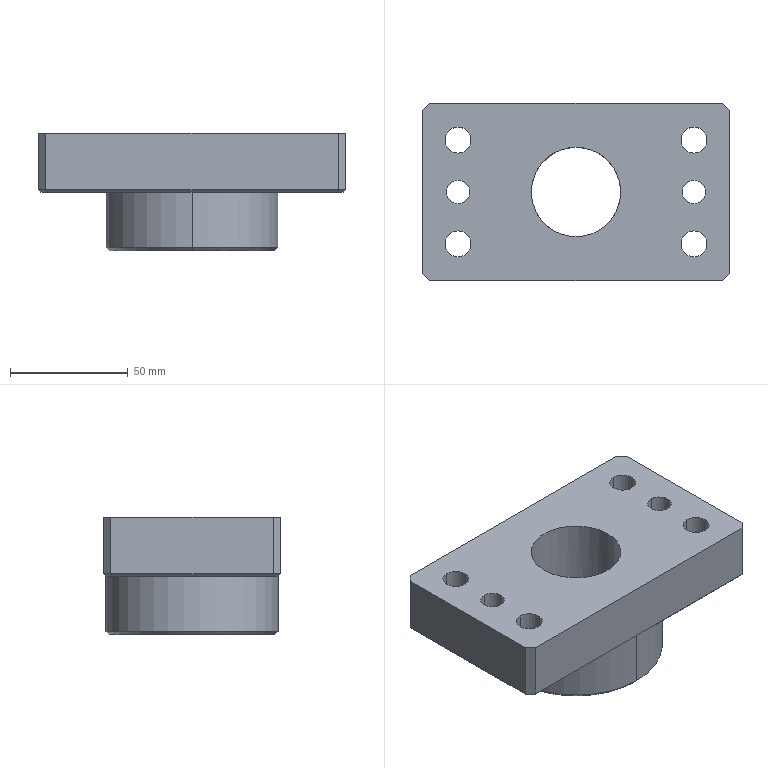Part | NX | features MYKP38-200_1 2 | 1 solid | 178 faces | box 130 x 75 x 50 mm | volume 277303 mm3 | plane 121 | cylinder 55 | cone 2 | commonest cylinder face diameters 11 x8 10 x4 3.991 x2 4.986 x2 5.223 x2 6.232 x2